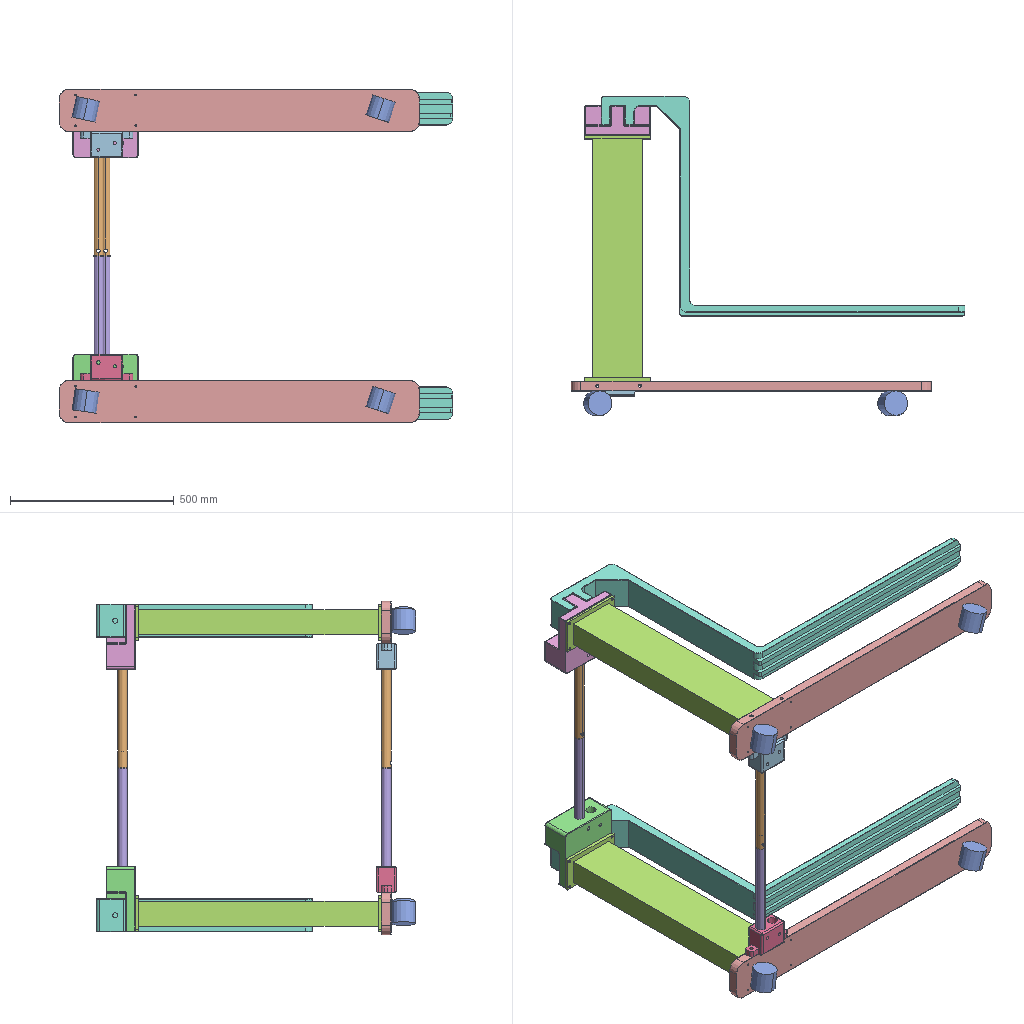Assembly | SolidWorks | 10 different items | 18 placed | box 1202 x 975 x 1019 mm
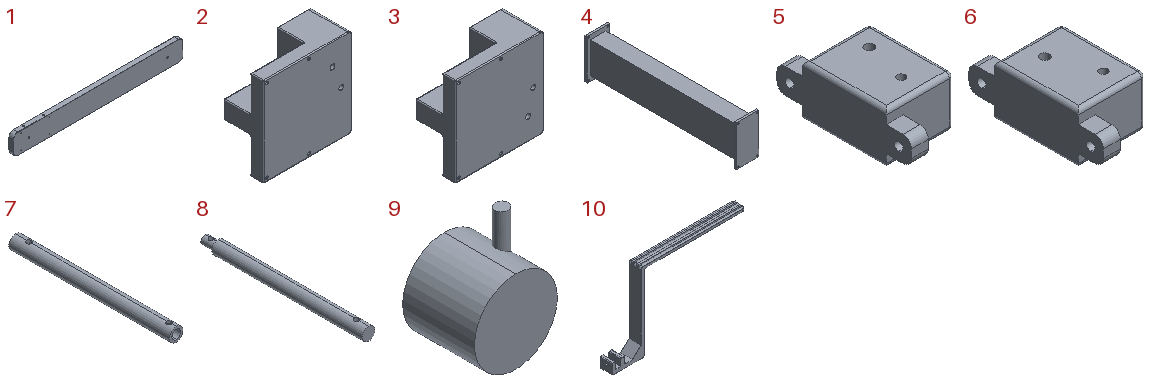Parts list (item | quantity | size | volume | features):
1 | x2 | 1100 x 30 x 130 mm | 4243037 mm3 | features HoleWzd 3, Chamfer 1, Extrusion 1, Fillet 1
2 | x1 | 200 x 90 x 200 mm | 2336478 mm3 | features ICE 8, Fillet 2, MoveFace 2, Extrusion 1, HoleWzd 1
3 | x1 | 200 x 90 x 200 mm | 2319927 mm3 | features ICE 7, Fillet 2, Extrusion 1, HoleWzd 1, MoveFace 1
4 | x2 | 110 x 750 x 200 mm | 9118663 mm3 | features ICE 2, Extrusion 1
5 | x1 | 80 x 160 x 60 mm | 411118 mm3 | features ICE 5, Extrusion 1, Fillet 1
6 | x1 | 80 x 160 x 60 mm | 411118 mm3 | features ICE 5, Extrusion 1, Fillet 1
7 | x2 | 30 x 354 x 30 mm | 230741 mm3 | features ICE 2, Extrusion 1, MoveFace 1
8 | x2 | 30 x 384 x 30 mm | 253782 mm3 | features ICE 2, MoveFace 2, Extrusion 1
9 | x4 | 75 x 65 x 102.5 mm | 290882 mm3 | features Extrusion 1, ICE 1
10 | x2 | 1110 x 100 x 669.85 mm | 5186013 mm3 | features Fillet 6, ICE 3, Chamfer 2, Extrusion 1, MoveFace 1
Mates (type | each side: item.copy, entity, surface, feature):
Coincident | 1.1 face plane Boss-Extrude1 | 4.1 face plane Boss-Extrude1
Concentric | 1.1 face cylinder M6 Tapped Hole1 | 4.1 face cylinder Boss-Extrude1 | 2 times
Concentric | 1.1 face cylinder M12 Tapped Hole1 | 9.1 face cylinder Boss-Extrude2
Tangent | 1.1 face plane Boss-Extrude1 | 9.1 face cylinder Boss-Extrude1
Concentric | 1.1 face cylinder M12 Tapped Hole1 | 9.2 face cylinder Boss-Extrude2
Tangent | 1.1 face plane Boss-Extrude1 | 9.2 face cylinder Boss-Extrude1
Concentric | 1.2 face cylinder M6 Tapped Hole1 | 4.2 face cylinder Boss-Extrude1 | 2 times
Concentric | 1.2 face cylinder M12 Tapped Hole1 | 9.3 face cylinder Boss-Extrude2
Concentric | 1.2 face cylinder M12 Tapped Hole1 | 9.4 face cylinder Boss-Extrude2
Tangent | 1.2 face plane Boss-Extrude1 | 9.3 face cylinder Boss-Extrude1
Coincident | 1.2 face plane Boss-Extrude1 | 4.2 face plane Boss-Extrude1
Tangent | 1.2 face plane Boss-Extrude1 | 9.4 face cylinder Boss-Extrude1
Coincident | 1.1 face plane Boss-Extrude1 | 1.2 face plane Boss-Extrude1 | 2 times
Coincident | 4.1 face plane Boss-Extrude4 | 2.1 face plane Boss-Extrude1 | 3 times
Concentric | 7.1 face cylinder Boss-Extrude1 | 2.1 face cylinder Cut-Extrude1
Concentric | 2.1 face cylinder Cut-Extrude2 | 7.1 face cylinder Cut-Extrude3
Concentric | 7.1 face cylinder Boss-Extrude1 | 8.1 face cylinder Boss-Extrude1
Coincident | 4.2 face plane Boss-Extrude4 | 3.1 face plane Boss-Extrude1 | 3 times
Coincident | 10.1 face plane Boss-Extrude1 | 3.1 face plane Boss-Extrude2
Coincident | 2.1 face plane Boss-Extrude2 | 10.2 face plane Boss-Extrude1
DistanceDim | 10.2 face plane Boss-Extrude1 | 2.1 face plane Boss-Extrude2
Coincident | 2.1 face plane Boss-Extrude1 | 10.2 face plane Boss-Extrude1
Coincident | 10.1 face plane Boss-Extrude1 | 3.1 face plane Boss-Extrude1
DistanceDim | 10.1 face plane Boss-Extrude1 | 3.1 face plane Boss-Extrude2
Coincident | 1.1 face plane Boss-Extrude1 | 6.1 face plane Boss-Extrude1
Concentric | 1.1 face cylinder M10 Tapped Hole1 | 6.1 face cylinder Boss-Extrude2 | 2 times
Coincident | 1.2 face plane Boss-Extrude1 | 5.1 face plane Boss-Extrude1
Concentric | 1.2 face cylinder M10 Tapped Hole1 | 5.1 face cylinder Boss-Extrude2 | 2 times
Concentric | 6.1 face cylinder Cut-Extrude1 | 7.2 face cylinder Boss-Extrude1
Concentric | 6.1 face cylinder Cut-Extrude3 | 7.2 face cylinder Cut-Extrude3
Concentric | 7.2 face cylinder Boss-Extrude1 | 8.2 face cylinder Boss-Extrude1
Concentric | 7.2 face cylinder Cut-Extrude3 | 8.2 face cylinder Cut-Extrude1